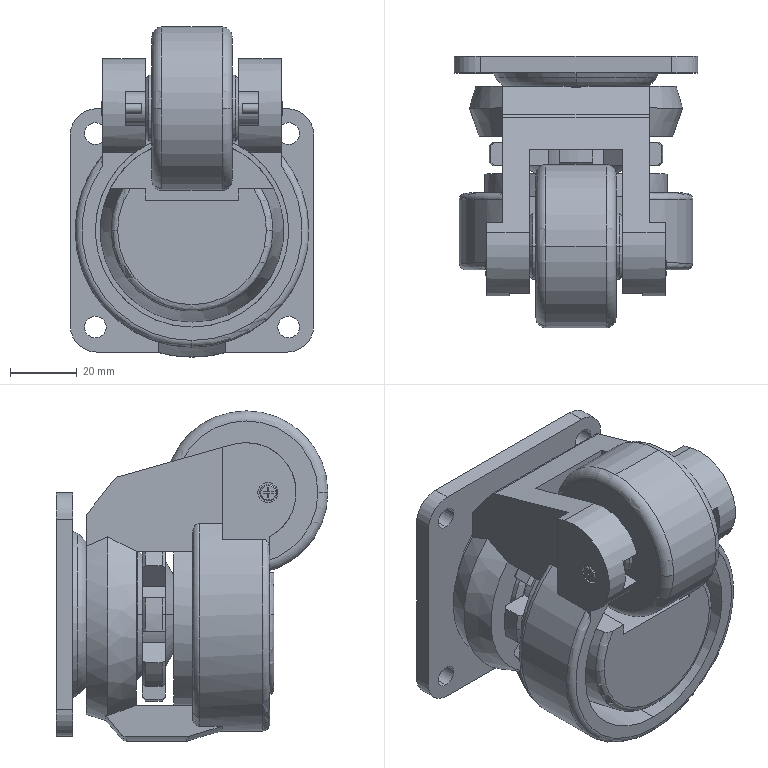Part | SolidWorks | features BaseBody 4 | 4 solids | 333 faces | box 73 x 81.5 x 99 mm | volume 238657 mm3 | plane 159 | cylinder 82 | cone 67 | torus 17 | spline 8 | commonest cylinder face diameters 52 x9 6.5 x8 10 x8 35 x8 3 x6 5 x4